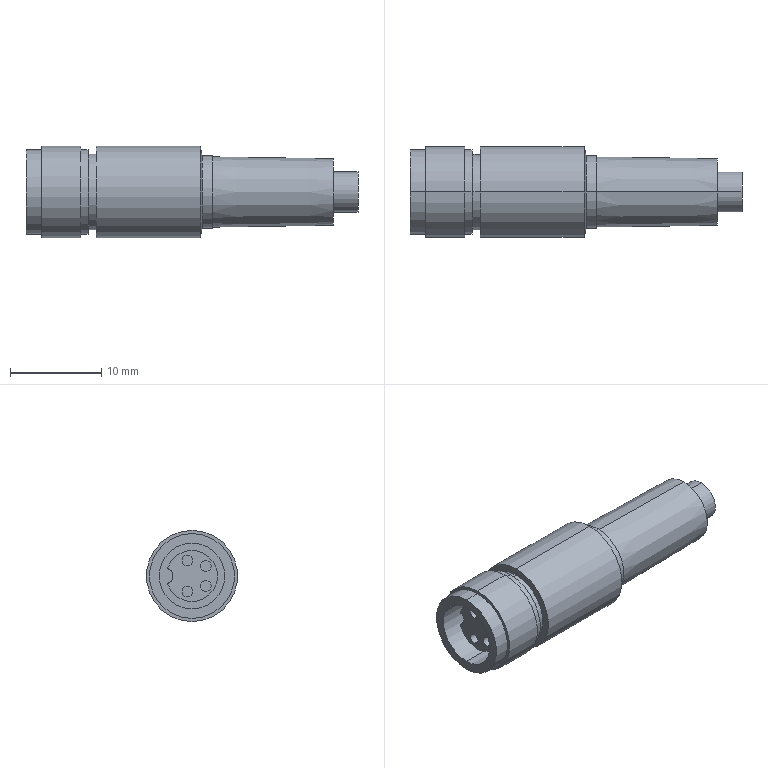Part | STEP file | OP-88071-Part-1 | 1 solid | 51 faces | box 36.4 x 10 x 10 mm | volume 1970 mm3 | cylinder 31 | plane 14 | cone 6 | commonest cylinder face diameters 1.2 x8 9.3 x4 10 x4 5.6 x3 0.4 x2 1 x2
STEP:
#1=CARTESIAN_POINT('',(1.7,-1.5,-1.7));
#2=VERTEX_POINT('',#1);
#3=CARTESIAN_POINT('',(1.7,-1.5,-0.5));
#4=VERTEX_POINT('',#3);
#5=CARTESIAN_POINT('',(1.7,-1.5,-1.1));
#6=DIRECTION('',(-1.,0.,0.));
#7=DIRECTION('',(0.,1.,0.));
#8=AXIS2_PLACEMENT_3D('',#5,#6,#7);
#9=CIRCLE('',#8,0.6);
#10=EDGE_CURVE('',#2,#4,#9,.T.);
#11=ORIENTED_EDGE('',*,*,#10,.T.);
#12=CARTESIAN_POINT('',(6.8,-1.5,-0.5));
#13=VERTEX_POINT('',#12);
#14=CARTESIAN_POINT('',(1.7,-1.5,-0.5));
#15=DIRECTION('',(1.,0.,0.));
#16=VECTOR('',#15,1000.);
#17=LINE('',#14,#16);
#18=EDGE_CURVE('',#4,#13,#17,.T.);
#19=ORIENTED_EDGE('',*,*,#18,.T.);
#20=CARTESIAN_POINT('',(6.8,-1.5,-1.7));
#21=VERTEX_POINT('',#20);
#22=CARTESIAN_POINT('',(6.8,-1.5,-1.1));
#23=DIRECTION('',(1.,0.,0.));
#24=DIRECTION('',(0.,0.,1.));
#25=AXIS2_PLACEMENT_3D('',#22,#23,#24);
#26=CIRCLE('',#25,0.6);
#27=EDGE_CURVE('',#13,#21,#26,.T.);
#28=ORIENTED_EDGE('',*,*,#27,.T.);
#29=CARTESIAN_POINT('',(1.7,-1.5,-1.7));
#30=DIRECTION('',(1.,0.,0.));
#31=VECTOR('',#30,1000.);
#32=LINE('',#29,#31);
#33=EDGE_CURVE('',#2,#21,#32,.T.);
#34=ORIENTED_EDGE('',*,*,#33,.F.);
#35=EDGE_LOOP('',(#11,#19,#28,#34));
#36=FACE_OUTER_BOUND('',#35,.T.);
#37=CARTESIAN_POINT('',(1.7,-1.5,-1.1));
#38=DIRECTION('',(1.,0.,0.));
#39=DIRECTION('',(0.,0.,-1.));
#40=AXIS2_PLACEMENT_3D('',#37,#38,#39);
#41=CYLINDRICAL_SURFACE('',#40,0.6);
#42=ADVANCED_FACE('',(#36),#41,.F.);
#43=CARTESIAN_POINT('',(1.7,-1.5,0.5));
#44=VERTEX_POINT('',#43);
#45=CARTESIAN_POINT('',(1.7,-1.5,1.7));
#46=VERTEX_POINT('',#45);
#47=CARTESIAN_POINT('',(1.7,-1.5,1.1));
#48=DIRECTION('',(-1.,0.,0.));
#49=DIRECTION('',(0.,1.,0.));
#50=AXIS2_PLACEMENT_3D('',#47,#48,#49);
#51=CIRCLE('',#50,0.6);
#52=EDGE_CURVE('',#44,#46,#51,.T.);
#53=ORIENTED_EDGE('',*,*,#52,.T.);
#54=CARTESIAN_POINT('',(6.8,-1.5,1.7));
#55=VERTEX_POINT('',#54);
#56=CARTESIAN_POINT('',(1.7,-1.5,1.7));
#57=DIRECTION('',(1.,0.,0.));
#58=VECTOR('',#57,1000.);
#59=LINE('',#56,#58);
#60=EDGE_CURVE('',#46,#55,#59,.T.);
#61=ORIENTED_EDGE('',*,*,#60,.T.);
#62=CARTESIAN_POINT('',(6.8,-1.5,0.5));
#63=VERTEX_POINT('',#62);
#64=CARTESIAN_POINT('',(6.8,-1.5,1.1));
#65=DIRECTION('',(1.,0.,0.));
#66=DIRECTION('',(0.,0.,1.));
#67=AXIS2_PLACEMENT_3D('',#64,#65,#66);
#68=CIRCLE('',#67,0.6);
#69=EDGE_CURVE('',#55,#63,#68,.T.);
#70=ORIENTED_EDGE('',*,*,#69,.T.);
#71=CARTESIAN_POINT('',(1.7,-1.5,0.5));
#72=DIRECTION('',(1.,0.,0.));
#73=VECTOR('',#72,1000.);
#74=LINE('',#71,#73);
#75=EDGE_CURVE('',#44,#63,#74,.T.);
#76=ORIENTED_EDGE('',*,*,#75,.F.);
#77=EDGE_LOOP('',(#53,#61,#70,#76));
#78=FACE_OUTER_BOUND('',#77,.T.);
#79=CARTESIAN_POINT('',(1.7,-1.5,1.1));
#80=DIRECTION('',(1.,0.,0.));
#81=DIRECTION('',(0.,0.,-1.));
#82=AXIS2_PLACEMENT_3D('',#79,#80,#81);
#83=CYLINDRICAL_SURFACE('',#82,0.6);
#84=ADVANCED_FACE('',(#78),#83,.F.);
#85=CARTESIAN_POINT('',(1.7,0.5,1.1));
#86=VERTEX_POINT('',#85);
#87=CARTESIAN_POINT('',(1.7,0.5,2.3));
#88=VERTEX_POINT('',#87);
#89=CARTESIAN_POINT('',(1.7,0.5,1.7));
#90=DIRECTION('',(-1.,0.,0.));
#91=DIRECTION('',(0.,1.,0.));
#92=AXIS2_PLACEMENT_3D('',#89,#90,#91);
#93=CIRCLE('',#92,0.6);
#94=EDGE_CURVE('',#86,#88,#93,.T.);
#95=ORIENTED_EDGE('',*,*,#94,.T.);
#96=CARTESIAN_POINT('',(6.8,0.5,2.3));
#97=VERTEX_POINT('',#96);
#98=CARTESIAN_POINT('',(1.7,0.5,2.3));
#99=DIRECTION('',(1.,0.,0.));
#100=VECTOR('',#99,1000.);
#101=LINE('',#98,#100);
#102=EDGE_CURVE('',#88,#97,#101,.T.);
#103=ORIENTED_EDGE('',*,*,#102,.T.);
#104=CARTESIAN_POINT('',(6.8,0.5,1.1));
#105=VERTEX_POINT('',#104);
#106=CARTESIAN_POINT('',(6.8,0.5,1.7));
#107=DIRECTION('',(1.,0.,0.));
#108=DIRECTION('',(0.,0.,1.));
#109=AXIS2_PLACEMENT_3D('',#106,#107,#108);
#110=CIRCLE('',#109,0.6);
#111=EDGE_CURVE('',#97,#105,#110,.T.);
#112=ORIENTED_EDGE('',*,*,#111,.T.);
#113=CARTESIAN_POINT('',(1.7,0.5,1.1));
#114=DIRECTION('',(1.,0.,0.));
#115=VECTOR('',#114,1000.);
#116=LINE('',#113,#115);
#117=EDGE_CURVE('',#86,#105,#116,.T.);
#118=ORIENTED_EDGE('',*,*,#117,.F.);
#119=EDGE_LOOP('',(#95,#103,#112,#118));
#120=FACE_OUTER_BOUND('',#119,.T.);
#121=CARTESIAN_POINT('',(1.7,0.5,1.7));
#122=DIRECTION('',(1.,0.,0.));
#123=DIRECTION('',(0.,0.,-1.));
#124=AXIS2_PLACEMENT_3D('',#121,#122,#123);
#125=CYLINDRICAL_SURFACE('',#124,0.6);
#126=ADVANCED_FACE('',(#120),#125,.F.);
#127=CARTESIAN_POINT('',(1.7,0.5,-2.3));
#128=VERTEX_POINT('',#127);
#129=CARTESIAN_POINT('',(1.7,0.5,-1.1));
#130=VERTEX_POINT('',#129);
#131=CARTESIAN_POINT('',(1.7,0.5,-1.7));
#132=DIRECTION('',(-1.,0.,0.));
#133=DIRECTION('',(0.,1.,0.));
#134=AXIS2_PLACEMENT_3D('',#131,#132,#133);
#135=CIRCLE('',#134,0.6);
#136=EDGE_CURVE('',#128,#130,#135,.T.);
#137=ORIENTED_EDGE('',*,*,#136,.T.);
#138=CARTESIAN_POINT('',(6.8,0.5,-1.1));
#139=VERTEX_POINT('',#138);
#140=CARTESIAN_POINT('',(1.7,0.5,-1.1));
#141=DIRECTION('',(1.,0.,0.));
#142=VECTOR('',#141,1000.);
#143=LINE('',#140,#142);
#144=EDGE_CURVE('',#130,#139,#143,.T.);
#145=ORIENTED_EDGE('',*,*,#144,.T.);
#146=CARTESIAN_POINT('',(6.8,0.5,-2.3));
#147=VERTEX_POINT('',#146);
#148=CARTESIAN_POINT('',(6.8,0.5,-1.7));
#149=DIRECTION('',(1.,0.,0.));
#150=DIRECTION('',(0.,0.,1.));
#151=AXIS2_PLACEMENT_3D('',#148,#149,#150);
#152=CIRCLE('',#151,0.6);
#153=EDGE_CURVE('',#139,#147,#152,.T.);
#154=ORIENTED_EDGE('',*,*,#153,.T.);
#155=CARTESIAN_POINT('',(1.7,0.5,-2.3));
#156=DIRECTION('',(1.,0.,0.));
#157=VECTOR('',#156,1000.);
#158=LINE('',#155,#157);
#159=EDGE_CURVE('',#128,#147,#158,.T.);
#160=ORIENTED_EDGE('',*,*,#159,.F.);
#161=EDGE_LOOP('',(#137,#145,#154,#160));
#162=FACE_OUTER_BOUND('',#161,.T.);
#163=CARTESIAN_POINT('',(1.7,0.5,-1.7));
#164=DIRECTION('',(1.,0.,0.));
#165=DIRECTION('',(0.,0.,-1.));
#166=AXIS2_PLACEMENT_3D('',#163,#164,#165);
#167=CYLINDRICAL_SURFACE('',#166,0.6);
#168=ADVANCED_FACE('',(#162),#167,.F.);
#169=CARTESIAN_POINT('',(1.7,0.,2.8));
#170=VERTEX_POINT('',#169);
#171=CARTESIAN_POINT('',(1.7,2.634,0.9507));
#172=VERTEX_POINT('',#171);
#173=CARTESIAN_POINT('',(1.7,0.,0.));
#174=DIRECTION('',(-1.,0.,0.));
#175=DIRECTION('',(0.,1.,0.));
#176=AXIS2_PLACEMENT_3D('',#173,#174,#175);
#177=CIRCLE('',#176,2.8);
#178=EDGE_CURVE('',#170,#172,#177,.T.);
#179=ORIENTED_EDGE('',*,*,#178,.F.);
#180=CARTESIAN_POINT('',(6.8,0.,2.8));
#181=VERTEX_POINT('',#180);
#182=CARTESIAN_POINT('',(1.7,0.,2.8));
#183=DIRECTION('',(1.,0.,0.));
#184=VECTOR('',#183,1000.);
#185=LINE('',#182,#184);
#186=EDGE_CURVE('',#170,#181,#185,.T.);
#187=ORIENTED_EDGE('',*,*,#186,.T.);
#188=CARTESIAN_POINT('',(6.8,2.634,0.9507));
#189=VERTEX_POINT('',#188);
#190=CARTESIAN_POINT('',(6.8,0.,0.));
#191=DIRECTION('',(-1.,0.,0.));
#192=DIRECTION('',(0.,1.,0.));
#193=AXIS2_PLACEMENT_3D('',#190,#191,#192);
#194=CIRCLE('',#193,2.8);
#195=EDGE_CURVE('',#181,#189,#194,.T.);
#196=ORIENTED_EDGE('',*,*,#195,.T.);
#197=CARTESIAN_POINT('',(1.7,2.634,0.9507));
#198=DIRECTION('',(1.,0.,0.));
#199=VECTOR('',#198,1000.);
#200=LINE('',#197,#199);
#201=EDGE_CURVE('',#172,#189,#200,.T.);
#202=ORIENTED_EDGE('',*,*,#201,.F.);
#203=EDGE_LOOP('',(#179,#187,#196,#202));
#204=FACE_OUTER_BOUND('',#203,.T.);
#205=CARTESIAN_POINT('',(1.7,0.,0.));
#206=DIRECTION('',(1.,0.,0.));
#207=DIRECTION('',(0.,0.,-1.));
#208=AXIS2_PLACEMENT_3D('',#205,#206,#207);
#209=CYLINDRICAL_SURFACE('',#208,2.8);
#210=ADVANCED_FACE('',(#204),#209,.T.);
#211=ORIENTED_EDGE('',*,*,#186,.F.);
#212=CARTESIAN_POINT('',(1.7,0.,-2.8));
#213=VERTEX_POINT('',#212);
#214=CARTESIAN_POINT('',(1.7,0.,0.));
#215=DIRECTION('',(-1.,0.,0.));
#216=DIRECTION('',(0.,1.,0.));
#217=AXIS2_PLACEMENT_3D('',#214,#215,#216);
#218=CIRCLE('',#217,2.8);
#219=EDGE_CURVE('',#213,#170,#218,.T.);
#220=ORIENTED_EDGE('',*,*,#219,.F.);
#221=CARTESIAN_POINT('',(6.8,0.,-2.8));
#222=VERTEX_POINT('',#221);
#223=CARTESIAN_POINT('',(1.7,0.,-2.8));
#224=DIRECTION('',(1.,0.,0.));
#225=VECTOR('',#224,1000.);
#226=LINE('',#223,#225);
#227=EDGE_CURVE('',#213,#222,#226,.T.);
#228=ORIENTED_EDGE('',*,*,#227,.T.);
#229=CARTESIAN_POINT('',(6.8,0.,0.));
#230=DIRECTION('',(-1.,0.,0.));
#231=DIRECTION('',(0.,1.,0.));
#232=AXIS2_PLACEMENT_3D('',#229,#230,#231);
#233=CIRCLE('',#232,2.8);
#234=EDGE_CURVE('',#222,#181,#233,.T.);
#235=ORIENTED_EDGE('',*,*,#234,.T.);
#236=EDGE_LOOP('',(#211,#220,#228,#235));
#237=FACE_OUTER_BOUND('',#236,.T.);
#238=CARTESIAN_POINT('',(1.7,0.,0.));
#239=DIRECTION('',(1.,0.,0.));
#240=DIRECTION('',(0.,0.,-1.));
#241=AXIS2_PLACEMENT_3D('',#238,#239,#240);
#242=CYLINDRICAL_SURFACE('',#241,2.8);
#243=ADVANCED_FACE('',(#237),#242,.T.);
#244=CARTESIAN_POINT('',(6.8,0.,-3.6));
#245=VERTEX_POINT('',#244);
#246=CARTESIAN_POINT('',(6.8,0.,3.6));
#247=VERTEX_POINT('',#246);
#248=CARTESIAN_POINT('',(6.8,0.,0.));
#249=DIRECTION('',(-1.,0.,0.));
#250=DIRECTION('',(0.,1.,0.));
#251=AXIS2_PLACEMENT_3D('',#248,#249,#250);
#252=CIRCLE('',#251,3.6);
#253=EDGE_CURVE('',#245,#247,#252,.T.);
#254=ORIENTED_EDGE('',*,*,#253,.F.);
#255=CARTESIAN_POINT('',(0.,0.,-3.6));
#256=VERTEX_POINT('',#255);
#257=CARTESIAN_POINT('',(6.8,0.,-3.6));
#258=DIRECTION('',(-1.,0.,0.));
#259=VECTOR('',#258,1000.);
#260=LINE('',#257,#259);
#261=EDGE_CURVE('',#245,#256,#260,.T.);
#262=ORIENTED_EDGE('',*,*,#261,.T.);
#263=CARTESIAN_POINT('',(0.,0.,3.6));
#264=VERTEX_POINT('',#263);
#265=CARTESIAN_POINT('',(0.,0.,0.));
#266=DIRECTION('',(-1.,0.,0.));
#267=DIRECTION('',(0.,1.,0.));
#268=AXIS2_PLACEMENT_3D('',#265,#266,#267);
#269=CIRCLE('',#268,3.6);
#270=EDGE_CURVE('',#256,#264,#269,.T.);
#271=ORIENTED_EDGE('',*,*,#270,.T.);
#272=CARTESIAN_POINT('',(6.8,0.,3.6));
#273=DIRECTION('',(-1.,0.,0.));
#274=VECTOR('',#273,1000.);
#275=LINE('',#272,#274);
#276=EDGE_CURVE('',#247,#264,#275,.T.);
#277=ORIENTED_EDGE('',*,*,#276,.F.);
#278=EDGE_LOOP('',(#254,#262,#271,#277));
#279=FACE_OUTER_BOUND('',#278,.T.);
#280=CARTESIAN_POINT('',(6.8,0.,0.));
#281=DIRECTION('',(-1.,0.,0.));
#282=DIRECTION('',(0.,0.,1.));
#283=AXIS2_PLACEMENT_3D('',#280,#281,#282);
#284=CYLINDRICAL_SURFACE('',#283,3.6);
#285=ADVANCED_FACE('',(#279),#284,.F.);
#286=CARTESIAN_POINT('',(33.7,0.,-2.2));
#287=VERTEX_POINT('',#286);
#288=CARTESIAN_POINT('',(33.7,0.,2.2));
#289=VERTEX_POINT('',#288);
#290=CARTESIAN_POINT('',(33.7,0.,0.));
#291=DIRECTION('',(1.,0.,0.));
#292=DIRECTION('',(0.,0.,-1.));
#293=AXIS2_PLACEMENT_3D('',#290,#291,#292);
#294=CIRCLE('',#293,2.2);
#295=EDGE_CURVE('',#287,#289,#294,.T.);
#296=ORIENTED_EDGE('',*,*,#295,.T.);
#297=CARTESIAN_POINT('',(36.4,0.,2.2));
#298=VERTEX_POINT('',#297);
#299=CARTESIAN_POINT('',(81.4,0.,2.2));
#300=DIRECTION('',(1.,0.,0.));
#301=VECTOR('',#300,1000.);
#302=LINE('',#299,#301);
#303=EDGE_CURVE('',#289,#298,#302,.T.);
#304=ORIENTED_EDGE('',*,*,#303,.T.);
#305=CARTESIAN_POINT('',(36.4,0.,-2.2));
#306=VERTEX_POINT('',#305);
#307=CARTESIAN_POINT('',(36.4,0.,0.));
#308=DIRECTION('',(1.,0.,0.));
#309=DIRECTION('',(0.,0.,-1.));
#310=AXIS2_PLACEMENT_3D('',#307,#308,#309);
#311=CIRCLE('',#310,2.2);
#312=EDGE_CURVE('',#306,#298,#311,.T.);
#313=ORIENTED_EDGE('',*,*,#312,.F.);
#314=CARTESIAN_POINT('',(81.4,0.,-2.2));
#315=DIRECTION('',(1.,0.,0.));
#316=VECTOR('',#315,1000.);
#317=LINE('',#314,#316);
#318=EDGE_CURVE('',#287,#306,#317,.T.);
#319=ORIENTED_EDGE('',*,*,#318,.F.);
#320=EDGE_LOOP('',(#296,#304,#313,#319));
#321=FACE_OUTER_BOUND('',#320,.T.);
#322=CARTESIAN_POINT('',(81.4,0.,0.));
#323=DIRECTION('',(1.,0.,0.));
#324=DIRECTION('',(0.,0.,-1.));
#325=AXIS2_PLACEMENT_3D('',#322,#323,#324);
#326=CYLINDRICAL_SURFACE('',#325,2.2);
#327=ADVANCED_FACE('',(#321),#326,.T.);
#328=CARTESIAN_POINT('',(33.7,0.,-3.65));
#329=VERTEX_POINT('',#328);
#330=CARTESIAN_POINT('',(33.7,0.,3.65));
#331=VERTEX_POINT('',#330);
#332=CARTESIAN_POINT('',(33.7,0.,0.));
#333=DIRECTION('',(1.,0.,0.));
#334=DIRECTION('',(0.,0.,-1.));
#335=AXIS2_PLACEMENT_3D('',#332,#333,#334);
#336=CIRCLE('',#335,3.65);
#337=EDGE_CURVE('',#329,#331,#336,.T.);
#338=ORIENTED_EDGE('',*,*,#337,.F.);
#339=CARTESIAN_POINT('',(20.4,0.,-3.85));
#340=VERTEX_POINT('',#339);
#341=CARTESIAN_POINT('',(20.4,0.,-3.85));
#342=DIRECTION('',(-0.9999,0.,-0.01504));
#343=VECTOR('',#342,1000.);
#344=LINE('',#341,#343);
#345=EDGE_CURVE('',#329,#340,#344,.T.);
#346=ORIENTED_EDGE('',*,*,#345,.T.);
#347=CARTESIAN_POINT('',(20.4,0.,3.85));
#348=VERTEX_POINT('',#347);
#349=CARTESIAN_POINT('',(20.4,0.,0.));
#350=DIRECTION('',(1.,0.,0.));
#351=DIRECTION('',(0.,0.,-1.));
#352=AXIS2_PLACEMENT_3D('',#349,#350,#351);
#353=CIRCLE('',#352,3.85);
#354=EDGE_CURVE('',#340,#348,#353,.T.);
#355=ORIENTED_EDGE('',*,*,#354,.T.);
#356=CARTESIAN_POINT('',(20.4,0.,3.85));
#357=DIRECTION('',(-0.9999,0.,0.01504));
#358=VECTOR('',#357,1000.);
#359=LINE('',#356,#358);
#360=EDGE_CURVE('',#331,#348,#359,.T.);
#361=ORIENTED_EDGE('',*,*,#360,.F.);
#362=EDGE_LOOP('',(#338,#346,#355,#361));
#363=FACE_OUTER_BOUND('',#362,.T.);
#364=CARTESIAN_POINT('',(20.4,0.,0.));
#365=DIRECTION('',(-1.,0.,0.));
#366=DIRECTION('',(0.,0.,1.));
#367=AXIS2_PLACEMENT_3D('',#364,#365,#366);
#368=CONICAL_SURFACE('',#367,3.85,0.01504);
#369=ADVANCED_FACE('',(#363),#368,.T.);
#370=CARTESIAN_POINT('',(19.3,0.,-4.));
#371=VERTEX_POINT('',#370);
#372=CARTESIAN_POINT('',(19.3,0.,4.));
#373=VERTEX_POINT('',#372);
#374=CARTESIAN_POINT('',(19.3,0.,0.));
#375=DIRECTION('',(1.,0.,0.));
#376=DIRECTION('',(0.,0.,-1.));
#377=AXIS2_PLACEMENT_3D('',#374,#375,#376);
#378=CIRCLE('',#377,4.);
#379=EDGE_CURVE('',#371,#373,#378,.T.);
#380=ORIENTED_EDGE('',*,*,#379,.T.);
#381=CARTESIAN_POINT('',(20.4,0.,4.));
#382=VERTEX_POINT('',#381);
#383=CARTESIAN_POINT('',(81.4,0.,4.));
#384=DIRECTION('',(1.,0.,0.));
#385=VECTOR('',#384,1000.);
#386=LINE('',#383,#385);
#387=EDGE_CURVE('',#373,#382,#386,.T.);
#388=ORIENTED_EDGE('',*,*,#387,.T.);
#389=CARTESIAN_POINT('',(20.4,0.,-4.));
#390=VERTEX_POINT('',#389);
#391=CARTESIAN_POINT('',(20.4,0.,0.));
#392=DIRECTION('',(1.,0.,0.));
#393=DIRECTION('',(0.,0.,-1.));
#394=AXIS2_PLACEMENT_3D('',#391,#392,#393);
#395=CIRCLE('',#394,4.);
#396=EDGE_CURVE('',#390,#382,#395,.T.);
#397=ORIENTED_EDGE('',*,*,#396,.F.);
#398=CARTESIAN_POINT('',(81.4,0.,-4.));
#399=DIRECTION('',(1.,0.,0.));
#400=VECTOR('',#399,1000.);
#401=LINE('',#398,#400);
#402=EDGE_CURVE('',#371,#390,#401,.T.);
#403=ORIENTED_EDGE('',*,*,#402,.F.);
#404=EDGE_LOOP('',(#380,#388,#397,#403));
#405=FACE_OUTER_BOUND('',#404,.T.);
#406=CARTESIAN_POINT('',(81.4,0.,0.));
#407=DIRECTION('',(1.,0.,0.));
#408=DIRECTION('',(0.,0.,-1.));
#409=AXIS2_PLACEMENT_3D('',#406,#407,#408);
#410=CYLINDRICAL_SURFACE('',#409,4.);
#411=ADVANCED_FACE('',(#405),#410,.T.);
#412=ORIENTED_EDGE('',*,*,#379,.F.);
#413=CARTESIAN_POINT('',(19.1,0.,-5.));
#414=VERTEX_POINT('',#413);
#415=CARTESIAN_POINT('',(19.1,0.,-5.));
#416=DIRECTION('',(-0.1961,0.,-0.9806));
#417=VECTOR('',#416,1000.);
#418=LINE('',#415,#417);
#419=EDGE_CURVE('',#371,#414,#418,.T.);
#420=ORIENTED_EDGE('',*,*,#419,.T.);
#421=CARTESIAN_POINT('',(19.1,0.,5.));
#422=VERTEX_POINT('',#421);
#423=CARTESIAN_POINT('',(19.1,0.,0.));
#424=DIRECTION('',(1.,0.,0.));
#425=DIRECTION('',(0.,0.,-1.));
#426=AXIS2_PLACEMENT_3D('',#423,#424,#425);
#427=CIRCLE('',#426,5.);
#428=EDGE_CURVE('',#414,#422,#427,.T.);
#429=ORIENTED_EDGE('',*,*,#428,.T.);
#430=CARTESIAN_POINT('',(19.1,0.,5.));
#431=DIRECTION('',(-0.1961,0.,0.9806));
#432=VECTOR('',#431,1000.);
#433=LINE('',#430,#432);
#434=EDGE_CURVE('',#373,#422,#433,.T.);
#435=ORIENTED_EDGE('',*,*,#434,.F.);
#436=EDGE_LOOP('',(#412,#420,#429,#435));
#437=FACE_OUTER_BOUND('',#436,.T.);
#438=CARTESIAN_POINT('',(19.1,0.,0.));
#439=DIRECTION('',(-1.,0.,0.));
#440=DIRECTION('',(0.,0.,1.));
#441=AXIS2_PLACEMENT_3D('',#438,#439,#440);
#442=CONICAL_SURFACE('',#441,5.,1.373);
#443=ADVANCED_FACE('',(#437),#442,.T.);
#444=CARTESIAN_POINT('',(7.7,0.,-5.));
#445=VERTEX_POINT('',#444);
#446=CARTESIAN_POINT('',(7.7,0.,5.));
#447=VERTEX_POINT('',#446);
#448=CARTESIAN_POINT('',(7.7,0.,0.));
#449=DIRECTION('',(1.,0.,0.));
#450=DIRECTION('',(0.,0.,-1.));
#451=AXIS2_PLACEMENT_3D('',#448,#449,#450);
#452=CIRCLE('',#451,5.);
#453=EDGE_CURVE('',#445,#447,#452,.T.);
#454=ORIENTED_EDGE('',*,*,#453,.T.);
#455=CARTESIAN_POINT('',(81.4,0.,5.));
#456=DIRECTION('',(1.,0.,0.));
#457=VECTOR('',#456,1000.);
#458=LINE('',#455,#457);
#459=EDGE_CURVE('',#447,#422,#458,.T.);
#460=ORIENTED_EDGE('',*,*,#459,.T.);
#461=ORIENTED_EDGE('',*,*,#428,.F.);
#462=CARTESIAN_POINT('',(81.4,0.,-5.));
#463=DIRECTION('',(1.,0.,0.));
#464=VECTOR('',#463,1000.);
#465=LINE('',#462,#464);
#466=EDGE_CURVE('',#445,#414,#465,.T.);
#467=ORIENTED_EDGE('',*,*,#466,.F.);
#468=EDGE_LOOP('',(#454,#460,#461,#467));
#469=FACE_OUTER_BOUND('',#468,.T.);
#470=CARTESIAN_POINT('',(81.4,0.,0.));
#471=DIRECTION('',(1.,0.,0.));
#472=DIRECTION('',(0.,0.,-1.));
#473=AXIS2_PLACEMENT_3D('',#470,#471,#472);
#474=CYLINDRICAL_SURFACE('',#473,5.);
#475=ADVANCED_FACE('',(#469),#474,.T.);
#476=CARTESIAN_POINT('',(6.9,0.,-4.15));
#477=VERTEX_POINT('',#476);
#478=CARTESIAN_POINT('',(6.9,0.,4.15));
#479=VERTEX_POINT('',#478);
#480=CARTESIAN_POINT('',(6.9,0.,0.));
#481=DIRECTION('',(1.,0.,0.));
#482=DIRECTION('',(0.,0.,-1.));
#483=AXIS2_PLACEMENT_3D('',#480,#481,#482);
#484=CIRCLE('',#483,4.15);
#485=EDGE_CURVE('',#477,#479,#484,.T.);
#486=ORIENTED_EDGE('',*,*,#485,.T.);
#487=CARTESIAN_POINT('',(7.7,0.,4.15));
#488=VERTEX_POINT('',#487);
#489=CARTESIAN_POINT('',(81.4,0.,4.15));
#490=DIRECTION('',(1.,0.,0.));
#491=VECTOR('',#490,1000.);
#492=LINE('',#489,#491);
#493=EDGE_CURVE('',#479,#488,#492,.T.);
#494=ORIENTED_EDGE('',*,*,#493,.T.);
#495=CARTESIAN_POINT('',(7.7,0.,-4.15));
#496=VERTEX_POINT('',#495);
#497=CARTESIAN_POINT('',(7.7,0.,0.));
#498=DIRECTION('',(1.,0.,0.));
#499=DIRECTION('',(0.,0.,-1.));
#500=AXIS2_PLACEMENT_3D('',#497,#498,#499);
#501=CIRCLE('',#500,4.15);
#502=EDGE_CURVE('',#496,#488,#501,.T.);
#503=ORIENTED_EDGE('',*,*,#502,.F.);
#504=CARTESIAN_POINT('',(81.4,0.,-4.15));
#505=DIRECTION('',(1.,0.,0.));
#506=VECTOR('',#505,1000.);
#507=LINE('',#504,#506);
#508=EDGE_CURVE('',#477,#496,#507,.T.);
#509=ORIENTED_EDGE('',*,*,#508,.F.);
#510=EDGE_LOOP('',(#486,#494,#503,#509));
#511=FACE_OUTER_BOUND('',#510,.T.);
#512=CARTESIAN_POINT('',(81.4,0.,0.));
#513=DIRECTION('',(1.,0.,0.));
#514=DIRECTION('',(0.,0.,-1.));
#515=AXIS2_PLACEMENT_3D('',#512,#513,#514);
#516=CYLINDRICAL_SURFACE('',#515,4.15);
#517=ADVANCED_FACE('',(#511),#516,.T.);
#518=ORIENTED_EDGE('',*,*,#485,.F.);
#519=CARTESIAN_POINT('',(6.8,0.,-4.65));
#520=VERTEX_POINT('',#519);
#521=CARTESIAN_POINT('',(6.8,0.,-4.65));
#522=DIRECTION('',(-0.1961,0.,-0.9806));
#523=VECTOR('',#522,1000.);
#524=LINE('',#521,#523);
#525=EDGE_CURVE('',#477,#520,#524,.T.);
#526=ORIENTED_EDGE('',*,*,#525,.T.);
#527=CARTESIAN_POINT('',(6.8,0.,4.65));
#528=VERTEX_POINT('',#527);
#529=CARTESIAN_POINT('',(6.8,0.,0.));
#530=DIRECTION('',(1.,0.,0.));
#531=DIRECTION('',(0.,0.,-1.));
#532=AXIS2_PLACEMENT_3D('',#529,#530,#531);
#533=CIRCLE('',#532,4.65);
#534=EDGE_CURVE('',#520,#528,#533,.T.);
#535=ORIENTED_EDGE('',*,*,#534,.T.);
#536=CARTESIAN_POINT('',(6.8,0.,4.65));
#537=DIRECTION('',(-0.1961,0.,0.9806));
#538=VECTOR('',#537,1000.);
#539=LINE('',#536,#538);
#540=EDGE_CURVE('',#479,#528,#539,.T.);
#541=ORIENTED_EDGE('',*,*,#540,.F.);
#542=EDGE_LOOP('',(#518,#526,#535,#541));
#543=FACE_OUTER_BOUND('',#542,.T.);
#544=CARTESIAN_POINT('',(6.8,0.,0.));
#545=DIRECTION('',(-1.,0.,0.));
#546=DIRECTION('',(0.,0.,1.));
#547=AXIS2_PLACEMENT_3D('',#544,#545,#546);
#548=CONICAL_SURFACE('',#547,4.65,1.373);
#549=ADVANCED_FACE('',(#543),#548,.T.);
#550=CARTESIAN_POINT('',(6.,0.,-4.65));
#551=VERTEX_POINT('',#550);
#552=CARTESIAN_POINT('',(6.,0.,4.65));
#553=VERTEX_POINT('',#552);
#554=CARTESIAN_POINT('',(6.,0.,0.));
#555=DIRECTION('',(1.,0.,0.));
#556=DIRECTION('',(0.,0.,-1.));
#557=AXIS2_PLACEMENT_3D('',#554,#555,#556);
#558=CIRCLE('',#557,4.65);
#559=EDGE_CURVE('',#551,#553,#558,.T.);
#560=ORIENTED_EDGE('',*,*,#559,.T.);
#561=CARTESIAN_POINT('',(81.4,0.,4.65));
#562=DIRECTION('',(1.,0.,0.));
#563=VECTOR('',#562,1000.);
#564=LINE('',#561,#563);
#565=EDGE_CURVE('',#553,#528,#564,.T.);
#566=ORIENTED_EDGE('',*,*,#565,.T.);
#567=ORIENTED_EDGE('',*,*,#534,.F.);
#568=CARTESIAN_POINT('',(81.4,0.,-4.65));
#569=DIRECTION('',(1.,0.,0.));
#570=VECTOR('',#569,1000.);
#571=LINE('',#568,#570);
#572=EDGE_CURVE('',#551,#520,#571,.T.);
#573=ORIENTED_EDGE('',*,*,#572,.F.);
#574=EDGE_LOOP('',(#560,#566,#567,#573));
#575=FACE_OUTER_BOUND('',#574,.T.);
#576=CARTESIAN_POINT('',(81.4,0.,0.));
#577=DIRECTION('',(1.,0.,0.));
#578=DIRECTION('',(0.,0.,-1.));
#579=AXIS2_PLACEMENT_3D('',#576,#577,#578);
#580=CYLINDRICAL_SURFACE('',#579,4.65);
#581=ADVANCED_FACE('',(#575),#580,.T.);
#582=CARTESIAN_POINT('',(1.7,0.,-5.));
#583=VERTEX_POINT('',#582);
#584=CARTESIAN_POINT('',(1.7,0.,5.));
#585=VERTEX_POINT('',#584);
#586=CARTESIAN_POINT('',(1.7,0.,0.));
#587=DIRECTION('',(1.,0.,0.));
#588=DIRECTION('',(0.,0.,-1.));
#589=AXIS2_PLACEMENT_3D('',#586,#587,#588);
#590=CIRCLE('',#589,5.);
#591=EDGE_CURVE('',#583,#585,#590,.T.);
#592=ORIENTED_EDGE('',*,*,#591,.T.);
#593=CARTESIAN_POINT('',(6.,0.,5.));
#594=VERTEX_POINT('',#593);
#595=CARTESIAN_POINT('',(81.4,0.,5.));
#596=DIRECTION('',(1.,0.,0.));
#597=VECTOR('',#596,1000.);
#598=LINE('',#595,#597);
#599=EDGE_CURVE('',#585,#594,#598,.T.);
#600=ORIENTED_EDGE('',*,*,#599,.T.);
#601=CARTESIAN_POINT('',(6.,0.,-5.));
#602=VERTEX_POINT('',#601);
#603=CARTESIAN_POINT('',(6.,0.,0.));
#604=DIRECTION('',(1.,0.,0.));
#605=DIRECTION('',(0.,0.,-1.));
#606=AXIS2_PLACEMENT_3D('',#603,#604,#605);
#607=CIRCLE('',#606,5.);
#608=EDGE_CURVE('',#602,#594,#607,.T.);
#609=ORIENTED_EDGE('',*,*,#608,.F.);
#610=CARTESIAN_POINT('',(81.4,0.,-5.));
#611=DIRECTION('',(1.,0.,0.));
#612=VECTOR('',#611,1000.);
#613=LINE('',#610,#612);
#614=EDGE_CURVE('',#583,#602,#613,.T.);
#615=ORIENTED_EDGE('',*,*,#614,.F.);
#616=EDGE_LOOP('',(#592,#600,#609,#615));
#617=FACE_OUTER_BOUND('',#616,.T.);
#618=CARTESIAN_POINT('',(81.4,0.,0.));
#619=DIRECTION('',(1.,0.,0.));
#620=DIRECTION('',(0.,0.,-1.));
#621=AXIS2_PLACEMENT_3D('',#618,#619,#620);
#622=CYLINDRICAL_SURFACE('',#621,5.);
#623=ADVANCED_FACE('',(#617),#622,.T.);
#624=CARTESIAN_POINT('',(0.,0.,-4.65));
#625=VERTEX_POINT('',#624);
#626=CARTESIAN_POINT('',(0.,0.,4.65));
#627=VERTEX_POINT('',#626);
#628=CARTESIAN_POINT('',(0.,0.,0.));
#629=DIRECTION('',(1.,0.,0.));
#630=DIRECTION('',(0.,0.,-1.));
#631=AXIS2_PLACEMENT_3D('',#628,#629,#630);
#632=CIRCLE('',#631,4.65);
#633=EDGE_CURVE('',#625,#627,#632,.T.);
#634=ORIENTED_EDGE('',*,*,#633,.T.);
#635=CARTESIAN_POINT('',(1.7,0.,4.65));
#636=VERTEX_POINT('',#635);
#637=CARTESIAN_POINT('',(81.4,0.,4.65));
#638=DIRECTION('',(1.,0.,0.));
#639=VECTOR('',#638,1000.);
#640=LINE('',#637,#639);
#641=EDGE_CURVE('',#627,#636,#640,.T.);
#642=ORIENTED_EDGE('',*,*,#641,.T.);
#643=CARTESIAN_POINT('',(1.7,0.,-4.65));
#644=VERTEX_POINT('',#643);
#645=CARTESIAN_POINT('',(1.7,0.,0.));
#646=DIRECTION('',(1.,0.,0.));
#647=DIRECTION('',(0.,0.,-1.));
#648=AXIS2_PLACEMENT_3D('',#645,#646,#647);
#649=CIRCLE('',#648,4.65);
#650=EDGE_CURVE('',#644,#636,#649,.T.);
#651=ORIENTED_EDGE('',*,*,#650,.F.);
#652=CARTESIAN_POINT('',(81.4,0.,-4.65));
#653=DIRECTION('',(1.,0.,0.));
#654=VECTOR('',#653,1000.);
#655=LINE('',#652,#654);
#656=EDGE_CURVE('',#625,#644,#655,.T.);
#657=ORIENTED_EDGE('',*,*,#656,.F.);
#658=EDGE_LOOP('',(#634,#642,#651,#657));
#659=FACE_OUTER_BOUND('',#658,.T.);
#660=CARTESIAN_POINT('',(81.4,0.,0.));
#661=DIRECTION('',(1.,0.,0.));
#662=DIRECTION('',(0.,0.,-1.));
#663=AXIS2_PLACEMENT_3D('',#660,#661,#662);
#664=CYLINDRICAL_SURFACE('',#663,4.65);
#665=ADVANCED_FACE('',(#659),#664,.T.);
#666=ORIENTED_EDGE('',*,*,#633,.F.);
#667=CARTESIAN_POINT('',(0.,0.,0.));
#668=DIRECTION('',(1.,0.,0.));
#669=DIRECTION('',(0.,0.,-1.));
#670=AXIS2_PLACEMENT_3D('',#667,#668,#669);
#671=CIRCLE('',#670,4.65);
#672=EDGE_CURVE('',#627,#625,#671,.T.);
#673=ORIENTED_EDGE('',*,*,#672,.F.);
#674=EDGE_LOOP('',(#666,#673));
#675=FACE_OUTER_BOUND('',#674,.T.);
#676=CARTESIAN_POINT('',(0.,0.,0.));
#677=DIRECTION('',(-1.,0.,0.));
#678=DIRECTION('',(0.,1.,0.));
#679=AXIS2_PLACEMENT_3D('',#676,#677,#678);
#680=CIRCLE('',#679,3.6);
#681=EDGE_CURVE('',#264,#256,#680,.T.);
#682=ORIENTED_EDGE('',*,*,#681,.F.);
#683=ORIENTED_EDGE('',*,*,#270,.F.);
#684=EDGE_LOOP('',(#682,#683));
#685=FACE_BOUND('',#684,.T.);
#686=CARTESIAN_POINT('',(0.,0.,0.));
#687=DIRECTION('',(1.,0.,0.));
#688=DIRECTION('',(0.,0.,-1.));
#689=AXIS2_PLACEMENT_3D('',#686,#687,#688);
#690=PLANE('',#689);
#691=ADVANCED_FACE('',(#675,#685),#690,.F.);
#692=ORIENTED_EDGE('',*,*,#641,.F.);
#693=ORIENTED_EDGE('',*,*,#672,.T.);
#694=ORIENTED_EDGE('',*,*,#656,.T.);
#695=CARTESIAN_POINT('',(1.7,0.,0.));
#696=DIRECTION('',(1.,0.,0.));
#697=DIRECTION('',(0.,0.,-1.));
#698=AXIS2_PLACEMENT_3D('',#695,#696,#697);
#699=CIRCLE('',#698,4.65);
#700=EDGE_CURVE('',#636,#644,#699,.T.);
#701=ORIENTED_EDGE('',*,*,#700,.F.);
#702=EDGE_LOOP('',(#692,#693,#694,#701));
#703=FACE_OUTER_BOUND('',#702,.T.);
#704=CARTESIAN_POINT('',(81.4,0.,0.));
#705=DIRECTION('',(1.,0.,0.));
#706=DIRECTION('',(0.,0.,-1.));
#707=AXIS2_PLACEMENT_3D('',#704,#705,#706);
#708=CYLINDRICAL_SURFACE('',#707,4.65);
#709=ADVANCED_FACE('',(#703),#708,.T.);
#710=ORIENTED_EDGE('',*,*,#591,.F.);
#711=CARTESIAN_POINT('',(1.7,0.,0.));
#712=DIRECTION('',(1.,0.,0.));
#713=DIRECTION('',(0.,0.,-1.));
#714=AXIS2_PLACEMENT_3D('',#711,#712,#713);
#715=CIRCLE('',#714,5.);
#716=EDGE_CURVE('',#585,#583,#715,.T.);
#717=ORIENTED_EDGE('',*,*,#716,.F.);
#718=EDGE_LOOP('',(#710,#717));
#719=FACE_OUTER_BOUND('',#718,.T.);
#720=ORIENTED_EDGE('',*,*,#650,.T.);
#721=ORIENTED_EDGE('',*,*,#700,.T.);
#722=EDGE_LOOP('',(#720,#721));
#723=FACE_BOUND('',#722,.T.);
#724=CARTESIAN_POINT('',(1.7,4.65,0.));
#725=DIRECTION('',(1.,0.,0.));
#726=DIRECTION('',(0.,0.,-1.));
#727=AXIS2_PLACEMENT_3D('',#724,#725,#726);
#728=PLANE('',#727);
#729=ADVANCED_FACE('',(#719,#723),#728,.F.);
#730=ORIENTED_EDGE('',*,*,#599,.F.);
#731=ORIENTED_EDGE('',*,*,#716,.T.);
#732=ORIENTED_EDGE('',*,*,#614,.T.);
#733=CARTESIAN_POINT('',(6.,0.,0.));
#734=DIRECTION('',(1.,0.,0.));
#735=DIRECTION('',(0.,0.,-1.));
#736=AXIS2_PLACEMENT_3D('',#733,#734,#735);
#737=CIRCLE('',#736,5.);
#738=EDGE_CURVE('',#594,#602,#737,.T.);
#739=ORIENTED_EDGE('',*,*,#738,.F.);
#740=EDGE_LOOP('',(#730,#731,#732,#739));
#741=FACE_OUTER_BOUND('',#740,.T.);
#742=CARTESIAN_POINT('',(81.4,0.,0.));
#743=DIRECTION('',(1.,0.,0.));
#744=DIRECTION('',(0.,0.,-1.));
#745=AXIS2_PLACEMENT_3D('',#742,#743,#744);
#746=CYLINDRICAL_SURFACE('',#745,5.);
#747=ADVANCED_FACE('',(#741),#746,.T.);
#748=ORIENTED_EDGE('',*,*,#559,.F.);
#749=CARTESIAN_POINT('',(6.,0.,0.));
#750=DIRECTION('',(1.,0.,0.));
#751=DIRECTION('',(0.,0.,-1.));
#752=AXIS2_PLACEMENT_3D('',#749,#750,#751);
#753=CIRCLE('',#752,4.65);
#754=EDGE_CURVE('',#553,#551,#753,.T.);
#755=ORIENTED_EDGE('',*,*,#754,.F.);
#756=EDGE_LOOP('',(#748,#755));
#757=FACE_BOUND('',#756,.T.);
#758=ORIENTED_EDGE('',*,*,#608,.T.);
#759=ORIENTED_EDGE('',*,*,#738,.T.);
#760=EDGE_LOOP('',(#758,#759));
#761=FACE_OUTER_BOUND('',#760,.T.);
#762=CARTESIAN_POINT('',(6.,5.,0.));
#763=DIRECTION('',(-1.,0.,0.));
#764=DIRECTION('',(0.,0.,1.));
#765=AXIS2_PLACEMENT_3D('',#762,#763,#764);
#766=PLANE('',#765);
#767=ADVANCED_FACE('',(#757,#761),#766,.F.);
#768=ORIENTED_EDGE('',*,*,#565,.F.);
#769=ORIENTED_EDGE('',*,*,#754,.T.);
#770=ORIENTED_EDGE('',*,*,#572,.T.);
#771=CARTESIAN_POINT('',(6.8,0.,0.));
#772=DIRECTION('',(1.,0.,0.));
#773=DIRECTION('',(0.,0.,-1.));
#774=AXIS2_PLACEMENT_3D('',#771,#772,#773);
#775=CIRCLE('',#774,4.65);
#776=EDGE_CURVE('',#528,#520,#775,.T.);
#777=ORIENTED_EDGE('',*,*,#776,.F.);
#778=EDGE_LOOP('',(#768,#769,#770,#777));
#779=FACE_OUTER_BOUND('',#778,.T.);
#780=CARTESIAN_POINT('',(81.4,0.,0.));
#781=DIRECTION('',(1.,0.,0.));
#782=DIRECTION('',(0.,0.,-1.));
#783=AXIS2_PLACEMENT_3D('',#780,#781,#782);
#784=CYLINDRICAL_SURFACE('',#783,4.65);
#785=ADVANCED_FACE('',(#779),#784,.T.);
#786=ORIENTED_EDGE('',*,*,#525,.F.);
#787=CARTESIAN_POINT('',(6.9,0.,0.));
#788=DIRECTION('',(1.,0.,0.));
#789=DIRECTION('',(0.,0.,-1.));
#790=AXIS2_PLACEMENT_3D('',#787,#788,#789);
#791=CIRCLE('',#790,4.15);
#792=EDGE_CURVE('',#479,#477,#791,.T.);
#793=ORIENTED_EDGE('',*,*,#792,.F.);
#794=ORIENTED_EDGE('',*,*,#540,.T.);
#795=ORIENTED_EDGE('',*,*,#776,.T.);
#796=EDGE_LOOP('',(#786,#793,#794,#795));
#797=FACE_OUTER_BOUND('',#796,.T.);
#798=CARTESIAN_POINT('',(6.8,0.,0.));
#799=DIRECTION('',(-1.,0.,0.));
#800=DIRECTION('',(0.,0.,1.));
#801=AXIS2_PLACEMENT_3D('',#798,#799,#800);
#802=CONICAL_SURFACE('',#801,4.65,1.373);
#803=ADVANCED_FACE('',(#797),#802,.T.);
#804=ORIENTED_EDGE('',*,*,#493,.F.);
#805=ORIENTED_EDGE('',*,*,#792,.T.);
#806=ORIENTED_EDGE('',*,*,#508,.T.);
#807=CARTESIAN_POINT('',(7.7,0.,0.));
#808=DIRECTION('',(1.,0.,0.));
#809=DIRECTION('',(0.,0.,-1.));
#810=AXIS2_PLACEMENT_3D('',#807,#808,#809);
#811=CIRCLE('',#810,4.15);
#812=EDGE_CURVE('',#488,#496,#811,.T.);
#813=ORIENTED_EDGE('',*,*,#812,.F.);
#814=EDGE_LOOP('',(#804,#805,#806,#813));
#815=FACE_OUTER_BOUND('',#814,.T.);
#816=CARTESIAN_POINT('',(81.4,0.,0.));
#817=DIRECTION('',(1.,0.,0.));
#818=DIRECTION('',(0.,0.,-1.));
#819=AXIS2_PLACEMENT_3D('',#816,#817,#818);
#820=CYLINDRICAL_SURFACE('',#819,4.15);
#821=ADVANCED_FACE('',(#815),#820,.T.);
#822=ORIENTED_EDGE('',*,*,#453,.F.);
#823=CARTESIAN_POINT('',(7.7,0.,0.));
#824=DIRECTION('',(1.,0.,0.));
#825=DIRECTION('',(0.,0.,-1.));
#826=AXIS2_PLACEMENT_3D('',#823,#824,#825);
#827=CIRCLE('',#826,5.);
#828=EDGE_CURVE('',#447,#445,#827,.T.);
#829=ORIENTED_EDGE('',*,*,#828,.F.);
#830=EDGE_LOOP('',(#822,#829));
#831=FACE_OUTER_BOUND('',#830,.T.);
#832=ORIENTED_EDGE('',*,*,#502,.T.);
#833=ORIENTED_EDGE('',*,*,#812,.T.);
#834=EDGE_LOOP('',(#832,#833));
#835=FACE_BOUND('',#834,.T.);
#836=CARTESIAN_POINT('',(7.7,4.15,0.));
#837=DIRECTION('',(1.,0.,0.));
#838=DIRECTION('',(0.,0.,-1.));
#839=AXIS2_PLACEMENT_3D('',#836,#837,#838);
#840=PLANE('',#839);
#841=ADVANCED_FACE('',(#831,#835),#840,.F.);
#842=ORIENTED_EDGE('',*,*,#459,.F.);
#843=ORIENTED_EDGE('',*,*,#828,.T.);
#844=ORIENTED_EDGE('',*,*,#466,.T.);
#845=CARTESIAN_POINT('',(19.1,0.,0.));
#846=DIRECTION('',(1.,0.,0.));
#847=DIRECTION('',(0.,0.,-1.));
#848=AXIS2_PLACEMENT_3D('',#845,#846,#847);
#849=CIRCLE('',#848,5.);
#850=EDGE_CURVE('',#422,#414,#849,.T.);
#851=ORIENTED_EDGE('',*,*,#850,.F.);
#852=EDGE_LOOP('',(#842,#843,#844,#851));
#853=FACE_OUTER_BOUND('',#852,.T.);
#854=CARTESIAN_POINT('',(81.4,0.,0.));
#855=DIRECTION('',(1.,0.,0.));
#856=DIRECTION('',(0.,0.,-1.));
#857=AXIS2_PLACEMENT_3D('',#854,#855,#856);
#858=CYLINDRICAL_SURFACE('',#857,5.);
#859=ADVANCED_FACE('',(#853),#858,.T.);
#860=ORIENTED_EDGE('',*,*,#419,.F.);
#861=CARTESIAN_POINT('',(19.3,0.,0.));
#862=DIRECTION('',(1.,0.,0.));
#863=DIRECTION('',(0.,0.,-1.));
#864=AXIS2_PLACEMENT_3D('',#861,#862,#863);
#865=CIRCLE('',#864,4.);
#866=EDGE_CURVE('',#373,#371,#865,.T.);
#867=ORIENTED_EDGE('',*,*,#866,.F.);
#868=ORIENTED_EDGE('',*,*,#434,.T.);
#869=ORIENTED_EDGE('',*,*,#850,.T.);
#870=EDGE_LOOP('',(#860,#867,#868,#869));
#871=FACE_OUTER_BOUND('',#870,.T.);
#872=CARTESIAN_POINT('',(19.1,0.,0.));
#873=DIRECTION('',(-1.,0.,0.));
#874=DIRECTION('',(0.,0.,1.));
#875=AXIS2_PLACEMENT_3D('',#872,#873,#874);
#876=CONICAL_SURFACE('',#875,5.,1.373);
#877=ADVANCED_FACE('',(#871),#876,.T.);
#878=ORIENTED_EDGE('',*,*,#387,.F.);
#879=ORIENTED_EDGE('',*,*,#866,.T.);
#880=ORIENTED_EDGE('',*,*,#402,.T.);
#881=CARTESIAN_POINT('',(20.4,0.,0.));
#882=DIRECTION('',(1.,0.,0.));
#883=DIRECTION('',(0.,0.,-1.));
#884=AXIS2_PLACEMENT_3D('',#881,#882,#883);
#885=CIRCLE('',#884,4.);
#886=EDGE_CURVE('',#382,#390,#885,.T.);
#887=ORIENTED_EDGE('',*,*,#886,.F.);
#888=EDGE_LOOP('',(#878,#879,#880,#887));
#889=FACE_OUTER_BOUND('',#888,.T.);
#890=CARTESIAN_POINT('',(81.4,0.,0.));
#891=DIRECTION('',(1.,0.,0.));
#892=DIRECTION('',(0.,0.,-1.));
#893=AXIS2_PLACEMENT_3D('',#890,#891,#892);
#894=CYLINDRICAL_SURFACE('',#893,4.);
#895=ADVANCED_FACE('',(#889),#894,.T.);
#896=CARTESIAN_POINT('',(20.4,0.,0.));
#897=DIRECTION('',(1.,0.,0.));
#898=DIRECTION('',(0.,0.,-1.));
#899=AXIS2_PLACEMENT_3D('',#896,#897,#898);
#900=CIRCLE('',#899,3.85);
#901=EDGE_CURVE('',#348,#340,#900,.T.);
#902=ORIENTED_EDGE('',*,*,#901,.F.);
#903=ORIENTED_EDGE('',*,*,#354,.F.);
#904=EDGE_LOOP('',(#902,#903));
#905=FACE_BOUND('',#904,.T.);
#906=ORIENTED_EDGE('',*,*,#396,.T.);
#907=ORIENTED_EDGE('',*,*,#886,.T.);
#908=EDGE_LOOP('',(#906,#907));
#909=FACE_OUTER_BOUND('',#908,.T.);
#910=CARTESIAN_POINT('',(20.4,4.,0.));
#911=DIRECTION('',(-1.,0.,0.));
#912=DIRECTION('',(0.,0.,1.));
#913=AXIS2_PLACEMENT_3D('',#910,#911,#912);
#914=PLANE('',#913);
#915=ADVANCED_FACE('',(#905,#909),#914,.F.);
#916=ORIENTED_EDGE('',*,*,#345,.F.);
#917=CARTESIAN_POINT('',(33.7,0.,0.));
#918=DIRECTION('',(1.,0.,0.));
#919=DIRECTION('',(0.,0.,-1.));
#920=AXIS2_PLACEMENT_3D('',#917,#918,#919);
#921=CIRCLE('',#920,3.65);
#922=EDGE_CURVE('',#331,#329,#921,.T.);
#923=ORIENTED_EDGE('',*,*,#922,.F.);
#924=ORIENTED_EDGE('',*,*,#360,.T.);
#925=ORIENTED_EDGE('',*,*,#901,.T.);
#926=EDGE_LOOP('',(#916,#923,#924,#925));
#927=FACE_OUTER_BOUND('',#926,.T.);
#928=CARTESIAN_POINT('',(20.4,0.,0.));
#929=DIRECTION('',(-1.,0.,0.));
#930=DIRECTION('',(0.,0.,1.));
#931=AXIS2_PLACEMENT_3D('',#928,#929,#930);
#932=CONICAL_SURFACE('',#931,3.85,0.01504);
#933=ADVANCED_FACE('',(#927),#932,.T.);
#934=ORIENTED_EDGE('',*,*,#295,.F.);
#935=CARTESIAN_POINT('',(33.7,0.,0.));
#936=DIRECTION('',(1.,0.,0.));
#937=DIRECTION('',(0.,0.,-1.));
#938=AXIS2_PLACEMENT_3D('',#935,#936,#937);
#939=CIRCLE('',#938,2.2);
#940=EDGE_CURVE('',#289,#287,#939,.T.);
#941=ORIENTED_EDGE('',*,*,#940,.F.);
#942=EDGE_LOOP('',(#934,#941));
#943=FACE_BOUND('',#942,.T.);
#944=ORIENTED_EDGE('',*,*,#922,.T.);
#945=ORIENTED_EDGE('',*,*,#337,.T.);
#946=EDGE_LOOP('',(#944,#945));
#947=FACE_OUTER_BOUND('',#946,.T.);
#948=CARTESIAN_POINT('',(33.7,3.65,0.));
#949=DIRECTION('',(-1.,0.,0.));
#950=DIRECTION('',(0.,0.,1.));
#951=AXIS2_PLACEMENT_3D('',#948,#949,#950);
#952=PLANE('',#951);
#953=ADVANCED_FACE('',(#943,#947),#952,.F.);
#954=ORIENTED_EDGE('',*,*,#303,.F.);
#955=ORIENTED_EDGE('',*,*,#940,.T.);
#956=ORIENTED_EDGE('',*,*,#318,.T.);
#957=CARTESIAN_POINT('',(36.4,0.,0.));
#958=DIRECTION('',(1.,0.,0.));
#959=DIRECTION('',(0.,0.,-1.));
#960=AXIS2_PLACEMENT_3D('',#957,#958,#959);
#961=CIRCLE('',#960,2.2);
#962=EDGE_CURVE('',#298,#306,#961,.T.);
#963=ORIENTED_EDGE('',*,*,#962,.F.);
#964=EDGE_LOOP('',(#954,#955,#956,#963));
#965=FACE_OUTER_BOUND('',#964,.T.);
#966=CARTESIAN_POINT('',(81.4,0.,0.));
#967=DIRECTION('',(1.,0.,0.));
#968=DIRECTION('',(0.,0.,-1.));
#969=AXIS2_PLACEMENT_3D('',#966,#967,#968);
#970=CYLINDRICAL_SURFACE('',#969,2.2);
#971=ADVANCED_FACE('',(#965),#970,.T.);
#972=ORIENTED_EDGE('',*,*,#312,.T.);
#973=ORIENTED_EDGE('',*,*,#962,.T.);
#974=EDGE_LOOP('',(#972,#973));
#975=FACE_OUTER_BOUND('',#974,.T.);
#976=CARTESIAN_POINT('',(36.4,2.2,0.));
#977=DIRECTION('',(-1.,0.,0.));
#978=DIRECTION('',(0.,0.,1.));
#979=AXIS2_PLACEMENT_3D('',#976,#977,#978);
#980=PLANE('',#979);
#981=ADVANCED_FACE('',(#975),#980,.F.);
#982=ORIENTED_EDGE('',*,*,#261,.F.);
#983=CARTESIAN_POINT('',(6.8,0.,0.));
#984=DIRECTION('',(-1.,0.,0.));
#985=DIRECTION('',(0.,1.,0.));
#986=AXIS2_PLACEMENT_3D('',#983,#984,#985);
#987=CIRCLE('',#986,3.6);
#988=EDGE_CURVE('',#247,#245,#987,.T.);
#989=ORIENTED_EDGE('',*,*,#988,.F.);
#990=ORIENTED_EDGE('',*,*,#276,.T.);
#991=ORIENTED_EDGE('',*,*,#681,.T.);
#992=EDGE_LOOP('',(#982,#989,#990,#991));
#993=FACE_OUTER_BOUND('',#992,.T.);
#994=CARTESIAN_POINT('',(6.8,0.,0.));
#995=DIRECTION('',(-1.,0.,0.));
#996=DIRECTION('',(0.,0.,1.));
#997=AXIS2_PLACEMENT_3D('',#994,#995,#996);
#998=CYLINDRICAL_SURFACE('',#997,3.6);
#999=ADVANCED_FACE('',(#993),#998,.F.);
#1000=CARTESIAN_POINT('',(6.8,2.634,-0.9507));
#1001=VERTEX_POINT('',#1000);
#1002=CARTESIAN_POINT('',(6.8,0.,0.));
#1003=DIRECTION('',(-1.,0.,0.));
#1004=DIRECTION('',(0.,1.,0.));
#1005=AXIS2_PLACEMENT_3D('',#1002,#1003,#1004);
#1006=CIRCLE('',#1005,2.8);
#1007=EDGE_CURVE('',#1001,#222,#1006,.T.);
#1008=ORIENTED_EDGE('',*,*,#1007,.F.);
#1009=CARTESIAN_POINT('',(6.8,2.49,-0.6877));
#1010=VERTEX_POINT('',#1009);
#1011=CARTESIAN_POINT('',(6.8,2.446,-0.8828));
#1012=DIRECTION('',(-1.,0.,0.));
#1013=DIRECTION('',(0.,1.,0.));
#1014=AXIS2_PLACEMENT_3D('',#1011,#1012,#1013);
#1015=CIRCLE('',#1014,0.2);
#1016=EDGE_CURVE('',#1010,#1001,#1015,.T.);
#1017=ORIENTED_EDGE('',*,*,#1016,.F.);
#1018=CARTESIAN_POINT('',(6.8,2.1,-0.2));
#1019=VERTEX_POINT('',#1018);
#1020=CARTESIAN_POINT('',(6.8,2.6,-0.2));
#1021=DIRECTION('',(-1.,0.,0.));
#1022=DIRECTION('',(0.,1.,0.));
#1023=AXIS2_PLACEMENT_3D('',#1020,#1021,#1022);
#1024=CIRCLE('',#1023,0.5);
#1025=EDGE_CURVE('',#1010,#1019,#1024,.T.);
#1026=ORIENTED_EDGE('',*,*,#1025,.T.);
#1027=CARTESIAN_POINT('',(6.8,2.1,0.2));
#1028=VERTEX_POINT('',#1027);
#1029=CARTESIAN_POINT('',(6.8,2.1,0.2));
#1030=DIRECTION('',(0.,0.,-1.));
#1031=VECTOR('',#1030,1000.);
#1032=LINE('',#1029,#1031);
#1033=EDGE_CURVE('',#1028,#1019,#1032,.T.);
#1034=ORIENTED_EDGE('',*,*,#1033,.F.);
#1035=CARTESIAN_POINT('',(6.8,2.49,0.6877));
#1036=VERTEX_POINT('',#1035);
#1037=CARTESIAN_POINT('',(6.8,2.6,0.2));
#1038=DIRECTION('',(-1.,0.,0.));
#1039=DIRECTION('',(0.,1.,0.));
#1040=AXIS2_PLACEMENT_3D('',#1037,#1038,#1039);
#1041=CIRCLE('',#1040,0.5);
#1042=EDGE_CURVE('',#1028,#1036,#1041,.T.);
#1043=ORIENTED_EDGE('',*,*,#1042,.T.);
#1044=CARTESIAN_POINT('',(6.8,2.446,0.8828));
#1045=DIRECTION('',(-1.,0.,0.));
#1046=DIRECTION('',(0.,1.,0.));
#1047=AXIS2_PLACEMENT_3D('',#1044,#1045,#1046);
#1048=CIRCLE('',#1047,0.2);
#1049=EDGE_CURVE('',#189,#1036,#1048,.T.);
#1050=ORIENTED_EDGE('',*,*,#1049,.F.);
#1051=ORIENTED_EDGE('',*,*,#195,.F.);
#1052=ORIENTED_EDGE('',*,*,#234,.F.);
#1053=EDGE_LOOP('',(#1008,#1017,#1026,#1034,#1043,#1050,#1051,#1052));
#1054=FACE_BOUND('',#1053,.T.);
#1055=ORIENTED_EDGE('',*,*,#988,.T.);
#1056=ORIENTED_EDGE('',*,*,#253,.T.);
#1057=EDGE_LOOP('',(#1055,#1056));
#1058=FACE_OUTER_BOUND('',#1057,.T.);
#1059=CARTESIAN_POINT('',(6.8,0.,0.));
#1060=DIRECTION('',(-1.,0.,0.));
#1061=DIRECTION('',(0.,0.,1.));
#1062=AXIS2_PLACEMENT_3D('',#1059,#1060,#1061);
#1063=PLANE('',#1062);
#1064=ADVANCED_FACE('',(#1054,#1058),#1063,.T.);
#1065=ORIENTED_EDGE('',*,*,#1016,.T.);
#1066=CARTESIAN_POINT('',(1.7,2.634,-0.9507));
#1067=VERTEX_POINT('',#1066);
#1068=CARTESIAN_POINT('',(1.7,2.634,-0.9507));
#1069=DIRECTION('',(1.,0.,0.));
#1070=VECTOR('',#1069,1000.);
#1071=LINE('',#1068,#1070);
#1072=EDGE_CURVE('',#1067,#1001,#1071,.T.);
#1073=ORIENTED_EDGE('',*,*,#1072,.F.);
#1074=CARTESIAN_POINT('',(1.7,2.49,-0.6877));
#1075=VERTEX_POINT('',#1074);
#1076=CARTESIAN_POINT('',(1.7,2.446,-0.8828));
#1077=DIRECTION('',(-1.,0.,0.));
#1078=DIRECTION('',(0.,1.,0.));
#1079=AXIS2_PLACEMENT_3D('',#1076,#1077,#1078);
#1080=CIRCLE('',#1079,0.2);
#1081=EDGE_CURVE('',#1075,#1067,#1080,.T.);
#1082=ORIENTED_EDGE('',*,*,#1081,.F.);
#1083=CARTESIAN_POINT('',(1.7,2.49,-0.6877));
#1084=DIRECTION('',(1.,0.,0.));
#1085=VECTOR('',#1084,1000.);
#1086=LINE('',#1083,#1085);
#1087=EDGE_CURVE('',#1075,#1010,#1086,.T.);
#1088=ORIENTED_EDGE('',*,*,#1087,.T.);
#1089=EDGE_LOOP('',(#1065,#1073,#1082,#1088));
#1090=FACE_OUTER_BOUND('',#1089,.T.);
#1091=CARTESIAN_POINT('',(1.7,2.446,-0.8828));
#1092=DIRECTION('',(1.,0.,0.));
#1093=DIRECTION('',(0.,0.,-1.));
#1094=AXIS2_PLACEMENT_3D('',#1091,#1092,#1093);
#1095=CYLINDRICAL_SURFACE('',#1094,0.2);
#1096=ADVANCED_FACE('',(#1090),#1095,.T.);
#1097=ORIENTED_EDGE('',*,*,#227,.F.);
#1098=CARTESIAN_POINT('',(1.7,0.,0.));
#1099=DIRECTION('',(-1.,0.,0.));
#1100=DIRECTION('',(0.,1.,0.));
#1101=AXIS2_PLACEMENT_3D('',#1098,#1099,#1100);
#1102=CIRCLE('',#1101,2.8);
#1103=EDGE_CURVE('',#1067,#213,#1102,.T.);
#1104=ORIENTED_EDGE('',*,*,#1103,.F.);
#1105=ORIENTED_EDGE('',*,*,#1072,.T.);
#1106=ORIENTED_EDGE('',*,*,#1007,.T.);
#1107=EDGE_LOOP('',(#1097,#1104,#1105,#1106));
#1108=FACE_OUTER_BOUND('',#1107,.T.);
#1109=CARTESIAN_POINT('',(1.7,0.,0.));
#1110=DIRECTION('',(1.,0.,0.));
#1111=DIRECTION('',(0.,0.,-1.));
#1112=AXIS2_PLACEMENT_3D('',#1109,#1110,#1111);
#1113=CYLINDRICAL_SURFACE('',#1112,2.8);
#1114=ADVANCED_FACE('',(#1108),#1113,.T.);
#1115=ORIENTED_EDGE('',*,*,#1049,.T.);
#1116=CARTESIAN_POINT('',(1.7,2.49,0.6877));
#1117=VERTEX_POINT('',#1116);
#1118=CARTESIAN_POINT('',(1.7,2.49,0.6877));
#1119=DIRECTION('',(1.,0.,0.));
#1120=VECTOR('',#1119,1000.);
#1121=LINE('',#1118,#1120);
#1122=EDGE_CURVE('',#1117,#1036,#1121,.T.);
#1123=ORIENTED_EDGE('',*,*,#1122,.F.);
#1124=CARTESIAN_POINT('',(1.7,2.446,0.8828));
#1125=DIRECTION('',(-1.,0.,0.));
#1126=DIRECTION('',(0.,1.,0.));
#1127=AXIS2_PLACEMENT_3D('',#1124,#1125,#1126);
#1128=CIRCLE('',#1127,0.2);
#1129=EDGE_CURVE('',#172,#1117,#1128,.T.);
#1130=ORIENTED_EDGE('',*,*,#1129,.F.);
#1131=ORIENTED_EDGE('',*,*,#201,.T.);
#1132=EDGE_LOOP('',(#1115,#1123,#1130,#1131));
#1133=FACE_OUTER_BOUND('',#1132,.T.);
#1134=CARTESIAN_POINT('',(1.7,2.446,0.8828));
#1135=DIRECTION('',(1.,0.,0.));
#1136=DIRECTION('',(0.,0.,-1.));
#1137=AXIS2_PLACEMENT_3D('',#1134,#1135,#1136);
#1138=CYLINDRICAL_SURFACE('',#1137,0.2);
#1139=ADVANCED_FACE('',(#1133),#1138,.T.);
#1140=ORIENTED_EDGE('',*,*,#1042,.F.);
#1141=CARTESIAN_POINT('',(1.7,2.1,0.2));
#1142=VERTEX_POINT('',#1141);
#1143=CARTESIAN_POINT('',(1.7,2.1,0.2));
#1144=DIRECTION('',(1.,0.,0.));
#1145=VECTOR('',#1144,1000.);
#1146=LINE('',#1143,#1145);
#1147=EDGE_CURVE('',#1142,#1028,#1146,.T.);
#1148=ORIENTED_EDGE('',*,*,#1147,.F.);
#1149=CARTESIAN_POINT('',(1.7,2.6,0.2));
#1150=DIRECTION('',(-1.,0.,0.));
#1151=DIRECTION('',(0.,1.,0.));
#1152=AXIS2_PLACEMENT_3D('',#1149,#1150,#1151);
#1153=CIRCLE('',#1152,0.5);
#1154=EDGE_CURVE('',#1142,#1117,#1153,.T.);
#1155=ORIENTED_EDGE('',*,*,#1154,.T.);
#1156=ORIENTED_EDGE('',*,*,#1122,.T.);
#1157=EDGE_LOOP('',(#1140,#1148,#1155,#1156));
#1158=FACE_OUTER_BOUND('',#1157,.T.);
#1159=CARTESIAN_POINT('',(1.7,2.6,0.2));
#1160=DIRECTION('',(1.,0.,0.));
#1161=DIRECTION('',(0.,0.,-1.));
#1162=AXIS2_PLACEMENT_3D('',#1159,#1160,#1161);
#1163=CYLINDRICAL_SURFACE('',#1162,0.5);
#1164=ADVANCED_FACE('',(#1158),#1163,.F.);
#1165=ORIENTED_EDGE('',*,*,#1033,.T.);
#1166=CARTESIAN_POINT('',(1.7,2.1,-0.2));
#1167=VERTEX_POINT('',#1166);
#1168=CARTESIAN_POINT('',(1.7,2.1,-0.2));
#1169=DIRECTION('',(1.,0.,0.));
#1170=VECTOR('',#1169,1000.);
#1171=LINE('',#1168,#1170);
#1172=EDGE_CURVE('',#1167,#1019,#1171,.T.);
#1173=ORIENTED_EDGE('',*,*,#1172,.F.);
#1174=CARTESIAN_POINT('',(1.7,2.1,0.2));
#1175=DIRECTION('',(0.,0.,-1.));
#1176=VECTOR('',#1175,1000.);
#1177=LINE('',#1174,#1176);
#1178=EDGE_CURVE('',#1142,#1167,#1177,.T.);
#1179=ORIENTED_EDGE('',*,*,#1178,.F.);
#1180=ORIENTED_EDGE('',*,*,#1147,.T.);
#1181=EDGE_LOOP('',(#1165,#1173,#1179,#1180));
#1182=FACE_OUTER_BOUND('',#1181,.T.);
#1183=CARTESIAN_POINT('',(1.7,2.1,0.2));
#1184=DIRECTION('',(0.,-1.,0.));
#1185=DIRECTION('',(0.,0.,-1.));
#1186=AXIS2_PLACEMENT_3D('',#1183,#1184,#1185);
#1187=PLANE('',#1186);
#1188=ADVANCED_FACE('',(#1182),#1187,.F.);
#1189=ORIENTED_EDGE('',*,*,#144,.F.);
#1190=CARTESIAN_POINT('',(1.7,0.5,-1.7));
#1191=DIRECTION('',(-1.,0.,0.));
#1192=DIRECTION('',(0.,1.,0.));
#1193=AXIS2_PLACEMENT_3D('',#1190,#1191,#1192);
#1194=CIRCLE('',#1193,0.6);
#1195=EDGE_CURVE('',#130,#128,#1194,.T.);
#1196=ORIENTED_EDGE('',*,*,#1195,.T.);
#1197=ORIENTED_EDGE('',*,*,#159,.T.);
#1198=CARTESIAN_POINT('',(6.8,0.5,-1.7));
#1199=DIRECTION('',(1.,0.,0.));
#1200=DIRECTION('',(0.,0.,1.));
#1201=AXIS2_PLACEMENT_3D('',#1198,#1199,#1200);
#1202=CIRCLE('',#1201,0.6);
#1203=EDGE_CURVE('',#147,#139,#1202,.T.);
#1204=ORIENTED_EDGE('',*,*,#1203,.T.);
#1205=EDGE_LOOP('',(#1189,#1196,#1197,#1204));
#1206=FACE_OUTER_BOUND('',#1205,.T.);
#1207=CARTESIAN_POINT('',(1.7,0.5,-1.7));
#1208=DIRECTION('',(1.,0.,0.));
#1209=DIRECTION('',(0.,0.,-1.));
#1210=AXIS2_PLACEMENT_3D('',#1207,#1208,#1209);
#1211=CYLINDRICAL_SURFACE('',#1210,0.6);
#1212=ADVANCED_FACE('',(#1206),#1211,.F.);
#1213=ORIENTED_EDGE('',*,*,#102,.F.);
#1214=CARTESIAN_POINT('',(1.7,0.5,1.7));
#1215=DIRECTION('',(-1.,0.,0.));
#1216=DIRECTION('',(0.,1.,0.));
#1217=AXIS2_PLACEMENT_3D('',#1214,#1215,#1216);
#1218=CIRCLE('',#1217,0.6);
#1219=EDGE_CURVE('',#88,#86,#1218,.T.);
#1220=ORIENTED_EDGE('',*,*,#1219,.T.);
#1221=ORIENTED_EDGE('',*,*,#117,.T.);
#1222=CARTESIAN_POINT('',(6.8,0.5,1.7));
#1223=DIRECTION('',(1.,0.,0.));
#1224=DIRECTION('',(0.,0.,1.));
#1225=AXIS2_PLACEMENT_3D('',#1222,#1223,#1224);
#1226=CIRCLE('',#1225,0.6);
#1227=EDGE_CURVE('',#105,#97,#1226,.T.);
#1228=ORIENTED_EDGE('',*,*,#1227,.T.);
#1229=EDGE_LOOP('',(#1213,#1220,#1221,#1228));
#1230=FACE_OUTER_BOUND('',#1229,.T.);
#1231=CARTESIAN_POINT('',(1.7,0.5,1.7));
#1232=DIRECTION('',(1.,0.,0.));
#1233=DIRECTION('',(0.,0.,-1.));
#1234=AXIS2_PLACEMENT_3D('',#1231,#1232,#1233);
#1235=CYLINDRICAL_SURFACE('',#1234,0.6);
#1236=ADVANCED_FACE('',(#1230),#1235,.F.);
#1237=ORIENTED_EDGE('',*,*,#60,.F.);
#1238=CARTESIAN_POINT('',(1.7,-1.5,1.1));
#1239=DIRECTION('',(-1.,0.,0.));
#1240=DIRECTION('',(0.,1.,0.));
#1241=AXIS2_PLACEMENT_3D('',#1238,#1239,#1240);
#1242=CIRCLE('',#1241,0.6);
#1243=EDGE_CURVE('',#46,#44,#1242,.T.);
#1244=ORIENTED_EDGE('',*,*,#1243,.T.);
#1245=ORIENTED_EDGE('',*,*,#75,.T.);
#1246=CARTESIAN_POINT('',(6.8,-1.5,1.1));
#1247=DIRECTION('',(1.,0.,0.));
#1248=DIRECTION('',(0.,0.,1.));
#1249=AXIS2_PLACEMENT_3D('',#1246,#1247,#1248);
#1250=CIRCLE('',#1249,0.6);
#1251=EDGE_CURVE('',#63,#55,#1250,.T.);
#1252=ORIENTED_EDGE('',*,*,#1251,.T.);
#1253=EDGE_LOOP('',(#1237,#1244,#1245,#1252));
#1254=FACE_OUTER_BOUND('',#1253,.T.);
#1255=CARTESIAN_POINT('',(1.7,-1.5,1.1));
#1256=DIRECTION('',(1.,0.,0.));
#1257=DIRECTION('',(0.,0.,-1.));
#1258=AXIS2_PLACEMENT_3D('',#1255,#1256,#1257);
#1259=CYLINDRICAL_SURFACE('',#1258,0.6);
#1260=ADVANCED_FACE('',(#1254),#1259,.F.);
#1261=ORIENTED_EDGE('',*,*,#18,.F.);
#1262=CARTESIAN_POINT('',(1.7,-1.5,-1.1));
#1263=DIRECTION('',(-1.,0.,0.));
#1264=DIRECTION('',(0.,1.,0.));
#1265=AXIS2_PLACEMENT_3D('',#1262,#1263,#1264);
#1266=CIRCLE('',#1265,0.6);
#1267=EDGE_CURVE('',#4,#2,#1266,.T.);
#1268=ORIENTED_EDGE('',*,*,#1267,.T.);
#1269=ORIENTED_EDGE('',*,*,#33,.T.);
#1270=CARTESIAN_POINT('',(6.8,-1.5,-1.1));
#1271=DIRECTION('',(1.,0.,0.));
#1272=DIRECTION('',(0.,0.,1.));
#1273=AXIS2_PLACEMENT_3D('',#1270,#1271,#1272);
#1274=CIRCLE('',#1273,0.6);
#1275=EDGE_CURVE('',#21,#13,#1274,.T.);
#1276=ORIENTED_EDGE('',*,*,#1275,.T.);
#1277=EDGE_LOOP('',(#1261,#1268,#1269,#1276));
#1278=FACE_OUTER_BOUND('',#1277,.T.);
#1279=CARTESIAN_POINT('',(1.7,-1.5,-1.1));
#1280=DIRECTION('',(1.,0.,0.));
#1281=DIRECTION('',(0.,0.,-1.));
#1282=AXIS2_PLACEMENT_3D('',#1279,#1280,#1281);
#1283=CYLINDRICAL_SURFACE('',#1282,0.6);
#1284=ADVANCED_FACE('',(#1278),#1283,.F.);
#1285=ORIENTED_EDGE('',*,*,#1025,.F.);
#1286=ORIENTED_EDGE('',*,*,#1087,.F.);
#1287=CARTESIAN_POINT('',(1.7,2.6,-0.2));
#1288=DIRECTION('',(-1.,0.,0.));
#1289=DIRECTION('',(0.,1.,0.));
#1290=AXIS2_PLACEMENT_3D('',#1287,#1288,#1289);
#1291=CIRCLE('',#1290,0.5);
#1292=EDGE_CURVE('',#1075,#1167,#1291,.T.);
#1293=ORIENTED_EDGE('',*,*,#1292,.T.);
#1294=ORIENTED_EDGE('',*,*,#1172,.T.);
#1295=EDGE_LOOP('',(#1285,#1286,#1293,#1294));
#1296=FACE_OUTER_BOUND('',#1295,.T.);
#1297=CARTESIAN_POINT('',(1.7,2.6,-0.2));
#1298=DIRECTION('',(1.,0.,0.));
#1299=DIRECTION('',(0.,0.,-1.));
#1300=AXIS2_PLACEMENT_3D('',#1297,#1298,#1299);
#1301=CYLINDRICAL_SURFACE('',#1300,0.5);
#1302=ADVANCED_FACE('',(#1296),#1301,.F.);
#1303=ORIENTED_EDGE('',*,*,#10,.F.);
#1304=ORIENTED_EDGE('',*,*,#1267,.F.);
#1305=EDGE_LOOP('',(#1303,#1304));
#1306=FACE_BOUND('',#1305,.T.);
#1307=ORIENTED_EDGE('',*,*,#52,.F.);
#1308=ORIENTED_EDGE('',*,*,#1243,.F.);
#1309=EDGE_LOOP('',(#1307,#1308));
#1310=FACE_BOUND('',#1309,.T.);
#1311=ORIENTED_EDGE('',*,*,#94,.F.);
#1312=ORIENTED_EDGE('',*,*,#1219,.F.);
#1313=EDGE_LOOP('',(#1311,#1312));
#1314=FACE_BOUND('',#1313,.T.);
#1315=ORIENTED_EDGE('',*,*,#136,.F.);
#1316=ORIENTED_EDGE('',*,*,#1195,.F.);
#1317=EDGE_LOOP('',(#1315,#1316));
#1318=FACE_BOUND('',#1317,.T.);
#1319=ORIENTED_EDGE('',*,*,#1081,.T.);
#1320=ORIENTED_EDGE('',*,*,#1103,.T.);
#1321=ORIENTED_EDGE('',*,*,#219,.T.);
#1322=ORIENTED_EDGE('',*,*,#178,.T.);
#1323=ORIENTED_EDGE('',*,*,#1129,.T.);
#1324=ORIENTED_EDGE('',*,*,#1154,.F.);
#1325=ORIENTED_EDGE('',*,*,#1178,.T.);
#1326=ORIENTED_EDGE('',*,*,#1292,.F.);
#1327=EDGE_LOOP('',(#1319,#1320,#1321,#1322,#1323,#1324,#1325,#1326));
#1328=FACE_OUTER_BOUND('',#1327,.T.);
#1329=CARTESIAN_POINT('',(1.7,2.446,-0.8828));
#1330=DIRECTION('',(-1.,0.,0.));
#1331=DIRECTION('',(0.,0.,1.));
#1332=AXIS2_PLACEMENT_3D('',#1329,#1330,#1331);
#1333=PLANE('',#1332);
#1334=ADVANCED_FACE('',(#1306,#1310,#1314,#1318,#1328),#1333,.T.);
#1335=ORIENTED_EDGE('',*,*,#1275,.F.);
#1336=ORIENTED_EDGE('',*,*,#27,.F.);
#1337=EDGE_LOOP('',(#1335,#1336));
#1338=FACE_OUTER_BOUND('',#1337,.T.);
#1339=CARTESIAN_POINT('',(6.8,0.,0.));
#1340=DIRECTION('',(-1.,0.,0.));
#1341=DIRECTION('',(0.,0.,1.));
#1342=AXIS2_PLACEMENT_3D('',#1339,#1340,#1341);
#1343=PLANE('',#1342);
#1344=ADVANCED_FACE('',(#1338),#1343,.T.);
#1345=ORIENTED_EDGE('',*,*,#1251,.F.);
#1346=ORIENTED_EDGE('',*,*,#69,.F.);
#1347=EDGE_LOOP('',(#1345,#1346));
#1348=FACE_OUTER_BOUND('',#1347,.T.);
#1349=CARTESIAN_POINT('',(6.8,0.,0.));
#1350=DIRECTION('',(-1.,0.,0.));
#1351=DIRECTION('',(0.,0.,1.));
#1352=AXIS2_PLACEMENT_3D('',#1349,#1350,#1351);
#1353=PLANE('',#1352);
#1354=ADVANCED_FACE('',(#1348),#1353,.T.);
#1355=ORIENTED_EDGE('',*,*,#1227,.F.);
#1356=ORIENTED_EDGE('',*,*,#111,.F.);
#1357=EDGE_LOOP('',(#1355,#1356));
#1358=FACE_OUTER_BOUND('',#1357,.T.);
#1359=CARTESIAN_POINT('',(6.8,0.,0.));
#1360=DIRECTION('',(-1.,0.,0.));
#1361=DIRECTION('',(0.,0.,1.));
#1362=AXIS2_PLACEMENT_3D('',#1359,#1360,#1361);
#1363=PLANE('',#1362);
#1364=ADVANCED_FACE('',(#1358),#1363,.T.);
#1365=ORIENTED_EDGE('',*,*,#1203,.F.);
#1366=ORIENTED_EDGE('',*,*,#153,.F.);
#1367=EDGE_LOOP('',(#1365,#1366));
#1368=FACE_OUTER_BOUND('',#1367,.T.);
#1369=CARTESIAN_POINT('',(6.8,0.,0.));
#1370=DIRECTION('',(-1.,0.,0.));
#1371=DIRECTION('',(0.,0.,1.));
#1372=AXIS2_PLACEMENT_3D('',#1369,#1370,#1371);
#1373=PLANE('',#1372);
#1374=ADVANCED_FACE('',(#1368),#1373,.T.);
#1375=CLOSED_SHELL('',(#42,#84,#126,#168,#210,#243,#285,#327,#369,#411,#443,#475,#517,#549,#581,#623,#665,#691,#709,#729,#747,#767,#785,#803,#821,#841,#859,#877,#895,#915,#933,#953,#971,#981,#999,#1064,#1096,#1114,#1139,#1164,#1188,#1212,#1236,#1260,#1284,#1302,#1334,#1344,#1354,#1364,#1374));
#1376=MANIFOLD_SOLID_BREP('',#1375);
#1377=CARTESIAN_POINT('',(0.,0.,0.));
#1378=DIRECTION('',(0.,0.,1.));
#1379=DIRECTION('',(1.,0.,0.));
#1380=AXIS2_PLACEMENT_3D('',#1377,#1378,#1379);
#1381=(LENGTH_UNIT()NAMED_UNIT(*)SI_UNIT(.MILLI.,.METRE.));
#1382=UNCERTAINTY_MEASURE_WITH_UNIT(LENGTH_MEASURE(0.00001),#1381,'','');
#1383=(NAMED_UNIT(*)PLANE_ANGLE_UNIT()SI_UNIT($,.RADIAN.));
#1384=(NAMED_UNIT(*)SI_UNIT($,.STERADIAN.)SOLID_ANGLE_UNIT());
#1385=(GEOMETRIC_REPRESENTATION_CONTEXT(3)GLOBAL_UNCERTAINTY_ASSIGNED_CONTEXT((#1382))GLOBAL_UNIT_ASSIGNED_CONTEXT((#1381,#1383,#1384))REPRESENTATION_CONTEXT('',''));
#1386=ADVANCED_BREP_SHAPE_REPRESENTATION('',(#1376,#1380),#1385);